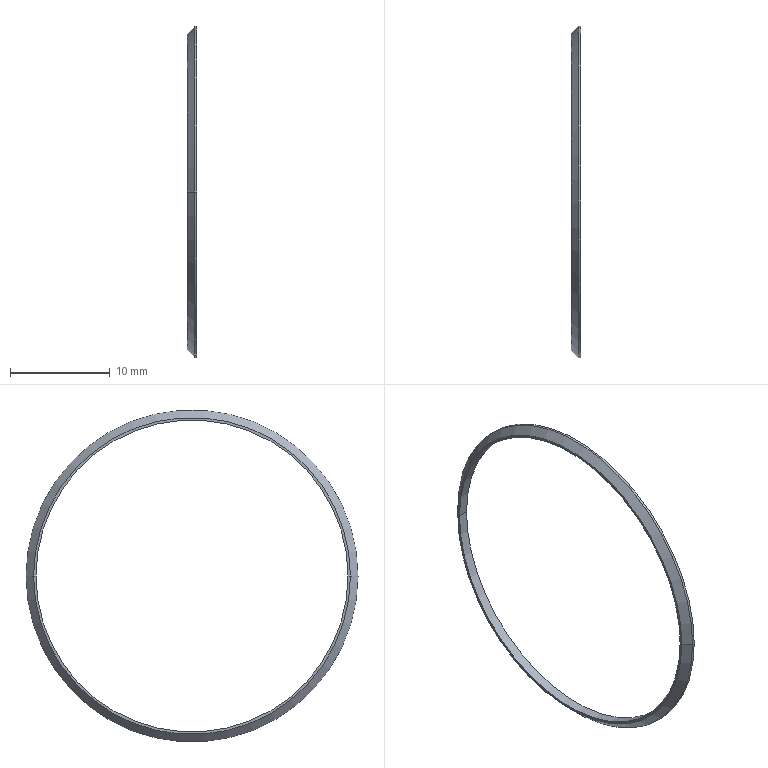Part | STEP file | BREP_7 | 1 solid | 10 faces | box 1 x 33.32 x 33.32 mm | volume 72.205 mm3 | plane 4 | cylinder 4 | cone 2 | commonest cylinder face diameters 31.311 x2 33.32 x2
STEP:
#1=CARTESIAN_POINT('',(0.,0.,0.));
#2=DIRECTION('',(0.,0.,1.));
#3=DIRECTION('',(1.,0.,0.));
#4=AXIS2_PLACEMENT_3D('',#1,#2,#3);
#5=CARTESIAN_POINT('',(-61.38,-16.66,0.));
#6=VERTEX_POINT('',#5);
#7=CARTESIAN_POINT('',(-61.38,-15.656,0.));
#8=VERTEX_POINT('',#7);
#9=CARTESIAN_POINT('',(-61.38,-16.66,0.));
#10=DIRECTION('',(0.,1.,0.));
#11=VECTOR('',#10,1.);
#12=LINE('',#9,#11);
#13=CARTESIAN_POINT('',(-61.38,0.,-16.158));
#14=DIRECTION('',(1.,0.,0.));
#15=DIRECTION('',(0.,-1.,0.));
#16=AXIS2_PLACEMENT_3D('',#13,#14,#15);
#17=PLANE('',#16);
#18=CARTESIAN_POINT('',(16.66,-16.158));
#19=DIRECTION('',(-1.,0.));
#20=VECTOR('',#19,1.);
#21=LINE('',#18,#20);
#22=(GEOMETRIC_REPRESENTATION_CONTEXT(2)PARAMETRIC_REPRESENTATION_CONTEXT()REPRESENTATION_CONTEXT('',''));
#23=DEFINITIONAL_REPRESENTATION('',(#21),#22);
#24=PCURVE('',#17,#23);
#25=CARTESIAN_POINT('',(-61.38,0.,16.158));
#26=DIRECTION('',(1.,0.,0.));
#27=DIRECTION('',(0.,1.,0.));
#28=AXIS2_PLACEMENT_3D('',#25,#26,#27);
#29=PLANE('',#28);
#30=CARTESIAN_POINT('',(-16.66,-16.158));
#31=DIRECTION('',(1.,0.));
#32=VECTOR('',#31,1.);
#33=LINE('',#30,#32);
#34=(GEOMETRIC_REPRESENTATION_CONTEXT(2)PARAMETRIC_REPRESENTATION_CONTEXT()REPRESENTATION_CONTEXT('',''));
#35=DEFINITIONAL_REPRESENTATION('',(#33),#34);
#36=PCURVE('',#29,#35);
#37=SURFACE_CURVE('',#12,(#24,#36),.PCURVE_S1.);
#38=EDGE_CURVE('',#6,#8,#37,.T.);
#39=ORIENTED_EDGE('',*,*,#38,.T.);
#40=CARTESIAN_POINT('',(-61.38,15.656,0.));
#41=VERTEX_POINT('',#40);
#42=CARTESIAN_POINT('',(-61.38,0.,0.));
#43=DIRECTION('',(-1.,0.,0.));
#44=DIRECTION('',(0.,1.,0.));
#45=AXIS2_PLACEMENT_3D('',#42,#43,#44);
#46=CIRCLE('',#45,15.656);
#47=CARTESIAN_POINT('',(-15.656,-16.158));
#48=CARTESIAN_POINT('',(-15.656,10.959));
#49=CARTESIAN_POINT('',(7.828,-2.6));
#50=CARTESIAN_POINT('',(31.311,-16.158));
#51=CARTESIAN_POINT('',(7.828,-29.716));
#52=CARTESIAN_POINT('',(-15.656,-43.274));
#53=CARTESIAN_POINT('',(-15.656,-16.158));
#54=(BOUNDED_CURVE()B_SPLINE_CURVE(2,(#47,#48,#49,#50,#51,#52,#53),.UNSPECIFIED.,.T.,.F.)B_SPLINE_CURVE_WITH_KNOTS((1,2,2,2,2,1),(-2.094,0.,2.094,4.189,6.283,8.378),.UNSPECIFIED.)CURVE()GEOMETRIC_REPRESENTATION_ITEM()RATIONAL_B_SPLINE_CURVE((1.,0.5,1.,0.5,1.,0.5,1.))REPRESENTATION_ITEM(''));
#55=(GEOMETRIC_REPRESENTATION_CONTEXT(2)PARAMETRIC_REPRESENTATION_CONTEXT()REPRESENTATION_CONTEXT('',''));
#56=DEFINITIONAL_REPRESENTATION('',(#54),#55);
#57=PCURVE('',#17,#56);
#58=CARTESIAN_POINT('',(-61.88,0.,0.));
#59=DIRECTION('',(1.,0.,0.));
#60=DIRECTION('',(0.,1.,0.));
#61=AXIS2_PLACEMENT_3D('',#58,#59,#60);
#62=CYLINDRICAL_SURFACE('',#61,15.656);
#63=CARTESIAN_POINT('',(6.283,0.5));
#64=DIRECTION('',(-1.,0.));
#65=VECTOR('',#64,1.);
#66=LINE('',#63,#65);
#67=(GEOMETRIC_REPRESENTATION_CONTEXT(2)PARAMETRIC_REPRESENTATION_CONTEXT()REPRESENTATION_CONTEXT('',''));
#68=DEFINITIONAL_REPRESENTATION('',(#66),#67);
#69=PCURVE('',#62,#68);
#70=SURFACE_CURVE('',#46,(#57,#69),.PCURVE_S1.);
#71=EDGE_CURVE('',#41,#8,#70,.T.);
#72=ORIENTED_EDGE('',*,*,#71,.F.);
#73=CARTESIAN_POINT('',(-61.38,16.66,0.));
#74=VERTEX_POINT('',#73);
#75=CARTESIAN_POINT('',(-61.38,16.66,0.));
#76=DIRECTION('',(0.,-1.,0.));
#77=VECTOR('',#76,1.);
#78=LINE('',#75,#77);
#79=CARTESIAN_POINT('',(-16.66,-16.158));
#80=DIRECTION('',(1.,0.));
#81=VECTOR('',#80,1.);
#82=LINE('',#79,#81);
#83=(GEOMETRIC_REPRESENTATION_CONTEXT(2)PARAMETRIC_REPRESENTATION_CONTEXT()REPRESENTATION_CONTEXT('',''));
#84=DEFINITIONAL_REPRESENTATION('',(#82),#83);
#85=PCURVE('',#17,#84);
#86=CARTESIAN_POINT('',(16.66,-16.158));
#87=DIRECTION('',(-1.,0.));
#88=VECTOR('',#87,1.);
#89=LINE('',#86,#88);
#90=(GEOMETRIC_REPRESENTATION_CONTEXT(2)PARAMETRIC_REPRESENTATION_CONTEXT()REPRESENTATION_CONTEXT('',''));
#91=DEFINITIONAL_REPRESENTATION('',(#89),#90);
#92=PCURVE('',#29,#91);
#93=SURFACE_CURVE('',#78,(#85,#92),.PCURVE_S1.);
#94=EDGE_CURVE('',#74,#41,#93,.T.);
#95=ORIENTED_EDGE('',*,*,#94,.F.);
#96=CARTESIAN_POINT('',(-61.38,0.,0.));
#97=DIRECTION('',(1.,0.,0.));
#98=DIRECTION('',(0.,-1.,0.));
#99=AXIS2_PLACEMENT_3D('',#96,#97,#98);
#100=CIRCLE('',#99,16.66);
#101=CARTESIAN_POINT('',(0.,-16.158));
#102=DIRECTION('',(1.,0.));
#103=AXIS2_PLACEMENT_2D('',#101,#102);
#104=CIRCLE('',#103,16.66);
#105=(GEOMETRIC_REPRESENTATION_CONTEXT(2)PARAMETRIC_REPRESENTATION_CONTEXT()REPRESENTATION_CONTEXT('',''));
#106=DEFINITIONAL_REPRESENTATION('',(#104),#105);
#107=PCURVE('',#17,#106);
#108=CARTESIAN_POINT('',(-61.5,0.,0.));
#109=DIRECTION('',(-1.,0.,0.));
#110=DIRECTION('',(0.,1.,0.));
#111=AXIS2_PLACEMENT_3D('',#108,#109,#110);
#112=CYLINDRICAL_SURFACE('',#111,16.66);
#113=CARTESIAN_POINT('',(3.142,-0.12));
#114=DIRECTION('',(-1.,0.));
#115=VECTOR('',#114,1.);
#116=LINE('',#113,#115);
#117=(GEOMETRIC_REPRESENTATION_CONTEXT(2)PARAMETRIC_REPRESENTATION_CONTEXT()REPRESENTATION_CONTEXT('',''));
#118=DEFINITIONAL_REPRESENTATION('',(#116),#117);
#119=PCURVE('',#112,#118);
#120=SURFACE_CURVE('',#100,(#107,#119),.PCURVE_S1.);
#121=EDGE_CURVE('',#6,#74,#120,.T.);
#122=ORIENTED_EDGE('',*,*,#121,.F.);
#123=EDGE_LOOP('',(#39,#72,#95,#122));
#124=FACE_BOUND('',#123,.F.);
#125=ADVANCED_FACE('',(#124),#17,.T.);
#126=CARTESIAN_POINT('',(-61.38,0.,0.));
#127=DIRECTION('',(-1.,0.,0.));
#128=DIRECTION('',(0.,-1.,0.));
#129=AXIS2_PLACEMENT_3D('',#126,#127,#128);
#130=CIRCLE('',#129,15.656);
#131=CARTESIAN_POINT('',(-15.656,-16.158));
#132=CARTESIAN_POINT('',(-15.656,10.959));
#133=CARTESIAN_POINT('',(7.828,-2.6));
#134=CARTESIAN_POINT('',(31.311,-16.158));
#135=CARTESIAN_POINT('',(7.828,-29.716));
#136=CARTESIAN_POINT('',(-15.656,-43.274));
#137=CARTESIAN_POINT('',(-15.656,-16.158));
#138=(BOUNDED_CURVE()B_SPLINE_CURVE(2,(#131,#132,#133,#134,#135,#136,#137),.UNSPECIFIED.,.T.,.F.)B_SPLINE_CURVE_WITH_KNOTS((1,2,2,2,2,1),(-2.094,0.,2.094,4.189,6.283,8.378),.UNSPECIFIED.)CURVE()GEOMETRIC_REPRESENTATION_ITEM()RATIONAL_B_SPLINE_CURVE((1.,0.5,1.,0.5,1.,0.5,1.))REPRESENTATION_ITEM(''));
#139=(GEOMETRIC_REPRESENTATION_CONTEXT(2)PARAMETRIC_REPRESENTATION_CONTEXT()REPRESENTATION_CONTEXT('',''));
#140=DEFINITIONAL_REPRESENTATION('',(#138),#139);
#141=PCURVE('',#29,#140);
#142=CARTESIAN_POINT('',(-61.88,0.,0.));
#143=DIRECTION('',(1.,0.,0.));
#144=DIRECTION('',(0.,-1.,0.));
#145=AXIS2_PLACEMENT_3D('',#142,#143,#144);
#146=CYLINDRICAL_SURFACE('',#145,15.656);
#147=CARTESIAN_POINT('',(6.283,0.5));
#148=DIRECTION('',(-1.,0.));
#149=VECTOR('',#148,1.);
#150=LINE('',#147,#149);
#151=(GEOMETRIC_REPRESENTATION_CONTEXT(2)PARAMETRIC_REPRESENTATION_CONTEXT()REPRESENTATION_CONTEXT('',''));
#152=DEFINITIONAL_REPRESENTATION('',(#150),#151);
#153=PCURVE('',#146,#152);
#154=SURFACE_CURVE('',#130,(#141,#153),.PCURVE_S1.);
#155=EDGE_CURVE('',#8,#41,#154,.T.);
#156=ORIENTED_EDGE('',*,*,#155,.F.);
#157=ORIENTED_EDGE('',*,*,#38,.F.);
#158=CARTESIAN_POINT('',(-61.38,0.,0.));
#159=DIRECTION('',(1.,0.,0.));
#160=DIRECTION('',(0.,1.,0.));
#161=AXIS2_PLACEMENT_3D('',#158,#159,#160);
#162=CIRCLE('',#161,16.66);
#163=CARTESIAN_POINT('',(0.,-16.158));
#164=DIRECTION('',(1.,0.));
#165=AXIS2_PLACEMENT_2D('',#163,#164);
#166=CIRCLE('',#165,16.66);
#167=(GEOMETRIC_REPRESENTATION_CONTEXT(2)PARAMETRIC_REPRESENTATION_CONTEXT()REPRESENTATION_CONTEXT('',''));
#168=DEFINITIONAL_REPRESENTATION('',(#166),#167);
#169=PCURVE('',#29,#168);
#170=CARTESIAN_POINT('',(-61.5,0.,0.));
#171=DIRECTION('',(-1.,0.,0.));
#172=DIRECTION('',(0.,-1.,0.));
#173=AXIS2_PLACEMENT_3D('',#170,#171,#172);
#174=CYLINDRICAL_SURFACE('',#173,16.66);
#175=CARTESIAN_POINT('',(3.142,-0.12));
#176=DIRECTION('',(-1.,0.));
#177=VECTOR('',#176,1.);
#178=LINE('',#175,#177);
#179=(GEOMETRIC_REPRESENTATION_CONTEXT(2)PARAMETRIC_REPRESENTATION_CONTEXT()REPRESENTATION_CONTEXT('',''));
#180=DEFINITIONAL_REPRESENTATION('',(#178),#179);
#181=PCURVE('',#174,#180);
#182=SURFACE_CURVE('',#162,(#169,#181),.PCURVE_S1.);
#183=EDGE_CURVE('',#74,#6,#182,.T.);
#184=ORIENTED_EDGE('',*,*,#183,.F.);
#185=ORIENTED_EDGE('',*,*,#94,.T.);
#186=EDGE_LOOP('',(#156,#157,#184,#185));
#187=FACE_BOUND('',#186,.F.);
#188=ADVANCED_FACE('',(#187),#29,.T.);
#189=CARTESIAN_POINT('',(-62.38,15.656,0.));
#190=VERTEX_POINT('',#189);
#191=CARTESIAN_POINT('',(-62.38,-15.656,0.));
#192=VERTEX_POINT('',#191);
#193=CARTESIAN_POINT('',(-62.38,0.,0.));
#194=DIRECTION('',(1.,0.,0.));
#195=DIRECTION('',(0.,1.,0.));
#196=AXIS2_PLACEMENT_3D('',#193,#194,#195);
#197=CIRCLE('',#196,15.656);
#198=CARTESIAN_POINT('',(3.142,-0.5));
#199=DIRECTION('',(1.,0.));
#200=VECTOR('',#199,1.);
#201=LINE('',#198,#200);
#202=(GEOMETRIC_REPRESENTATION_CONTEXT(2)PARAMETRIC_REPRESENTATION_CONTEXT()REPRESENTATION_CONTEXT('',''));
#203=DEFINITIONAL_REPRESENTATION('',(#201),#202);
#204=PCURVE('',#146,#203);
#205=CARTESIAN_POINT('',(-62.38,0.,15.778));
#206=DIRECTION('',(1.,0.,0.));
#207=DIRECTION('',(0.,1.,0.));
#208=AXIS2_PLACEMENT_3D('',#205,#206,#207);
#209=PLANE('',#208);
#210=CARTESIAN_POINT('',(0.,-15.778));
#211=DIRECTION('',(1.,0.));
#212=AXIS2_PLACEMENT_2D('',#210,#211);
#213=CIRCLE('',#212,15.656);
#214=(GEOMETRIC_REPRESENTATION_CONTEXT(2)PARAMETRIC_REPRESENTATION_CONTEXT()REPRESENTATION_CONTEXT('',''));
#215=DEFINITIONAL_REPRESENTATION('',(#213),#214);
#216=PCURVE('',#209,#215);
#217=SURFACE_CURVE('',#197,(#204,#216),.PCURVE_S1.);
#218=EDGE_CURVE('',#190,#192,#217,.T.);
#219=ORIENTED_EDGE('',*,*,#218,.T.);
#220=CARTESIAN_POINT('',(-61.38,-15.656,0.));
#221=DIRECTION('',(-1.,0.,0.));
#222=VECTOR('',#221,1.);
#223=LINE('',#220,#222);
#224=CARTESIAN_POINT('',(6.283,0.5));
#225=DIRECTION('',(0.,-1.));
#226=VECTOR('',#225,1.);
#227=LINE('',#224,#226);
#228=(GEOMETRIC_REPRESENTATION_CONTEXT(2)PARAMETRIC_REPRESENTATION_CONTEXT()REPRESENTATION_CONTEXT('',''));
#229=DEFINITIONAL_REPRESENTATION('',(#227),#228);
#230=PCURVE('',#146,#229);
#231=CARTESIAN_POINT('',(3.142,0.5));
#232=DIRECTION('',(0.,-1.));
#233=VECTOR('',#232,1.);
#234=LINE('',#231,#233);
#235=(GEOMETRIC_REPRESENTATION_CONTEXT(2)PARAMETRIC_REPRESENTATION_CONTEXT()REPRESENTATION_CONTEXT('',''));
#236=DEFINITIONAL_REPRESENTATION('',(#234),#235);
#237=PCURVE('',#62,#236);
#238=SURFACE_CURVE('',#223,(#230,#237),.PCURVE_S1.);
#239=EDGE_CURVE('',#8,#192,#238,.T.);
#240=ORIENTED_EDGE('',*,*,#239,.F.);
#241=ORIENTED_EDGE('',*,*,#155,.T.);
#242=CARTESIAN_POINT('',(-61.38,15.656,0.));
#243=DIRECTION('',(-1.,0.,0.));
#244=VECTOR('',#243,1.);
#245=LINE('',#242,#244);
#246=CARTESIAN_POINT('',(3.142,0.5));
#247=DIRECTION('',(0.,-1.));
#248=VECTOR('',#247,1.);
#249=LINE('',#246,#248);
#250=(GEOMETRIC_REPRESENTATION_CONTEXT(2)PARAMETRIC_REPRESENTATION_CONTEXT()REPRESENTATION_CONTEXT('',''));
#251=DEFINITIONAL_REPRESENTATION('',(#249),#250);
#252=PCURVE('',#146,#251);
#253=CARTESIAN_POINT('',(6.283,0.5));
#254=DIRECTION('',(0.,-1.));
#255=VECTOR('',#254,1.);
#256=LINE('',#253,#255);
#257=(GEOMETRIC_REPRESENTATION_CONTEXT(2)PARAMETRIC_REPRESENTATION_CONTEXT()REPRESENTATION_CONTEXT('',''));
#258=DEFINITIONAL_REPRESENTATION('',(#256),#257);
#259=PCURVE('',#62,#258);
#260=SURFACE_CURVE('',#245,(#252,#259),.PCURVE_S1.);
#261=EDGE_CURVE('',#41,#190,#260,.T.);
#262=ORIENTED_EDGE('',*,*,#261,.T.);
#263=EDGE_LOOP('',(#219,#240,#241,#262));
#264=FACE_BOUND('',#263,.F.);
#265=ADVANCED_FACE('',(#264),#146,.F.);
#266=CARTESIAN_POINT('',(-62.38,-15.9,0.));
#267=VERTEX_POINT('',#266);
#268=CARTESIAN_POINT('',(-62.38,15.9,0.));
#269=VERTEX_POINT('',#268);
#270=CARTESIAN_POINT('',(-62.38,0.,0.));
#271=DIRECTION('',(-1.,0.,0.));
#272=DIRECTION('',(0.,-1.,0.));
#273=AXIS2_PLACEMENT_3D('',#270,#271,#272);
#274=CIRCLE('',#273,15.9);
#275=CARTESIAN_POINT('',(-15.9,-15.778));
#276=CARTESIAN_POINT('',(-15.9,11.762));
#277=CARTESIAN_POINT('',(7.95,-2.008));
#278=CARTESIAN_POINT('',(31.8,-15.778));
#279=CARTESIAN_POINT('',(7.95,-29.548));
#280=CARTESIAN_POINT('',(-15.9,-43.317));
#281=CARTESIAN_POINT('',(-15.9,-15.778));
#282=(BOUNDED_CURVE()B_SPLINE_CURVE(2,(#275,#276,#277,#278,#279,#280,#281),.UNSPECIFIED.,.T.,.F.)B_SPLINE_CURVE_WITH_KNOTS((1,2,2,2,2,1),(-2.094,0.,2.094,4.189,6.283,8.378),.UNSPECIFIED.)CURVE()GEOMETRIC_REPRESENTATION_ITEM()RATIONAL_B_SPLINE_CURVE((1.,0.5,1.,0.5,1.,0.5,1.))REPRESENTATION_ITEM(''));
#283=(GEOMETRIC_REPRESENTATION_CONTEXT(2)PARAMETRIC_REPRESENTATION_CONTEXT()REPRESENTATION_CONTEXT('',''));
#284=DEFINITIONAL_REPRESENTATION('',(#282),#283);
#285=PCURVE('',#209,#284);
#286=CARTESIAN_POINT('',(-62.,0.,0.));
#287=DIRECTION('',(1.,0.,0.));
#288=DIRECTION('',(0.,1.,0.));
#289=AXIS2_PLACEMENT_3D('',#286,#287,#288);
#290=CONICAL_SURFACE('',#289,16.28,0.7854);
#291=CARTESIAN_POINT('',(3.142,-0.38));
#292=DIRECTION('',(-1.,0.));
#293=VECTOR('',#292,1.);
#294=LINE('',#291,#293);
#295=(GEOMETRIC_REPRESENTATION_CONTEXT(2)PARAMETRIC_REPRESENTATION_CONTEXT()REPRESENTATION_CONTEXT('',''));
#296=DEFINITIONAL_REPRESENTATION('',(#294),#295);
#297=PCURVE('',#290,#296);
#298=SURFACE_CURVE('',#274,(#285,#297),.PCURVE_S1.);
#299=EDGE_CURVE('',#267,#269,#298,.T.);
#300=ORIENTED_EDGE('',*,*,#299,.F.);
#301=CARTESIAN_POINT('',(-62.38,-15.656,0.));
#302=DIRECTION('',(0.,-1.,0.));
#303=VECTOR('',#302,1.);
#304=LINE('',#301,#303);
#305=CARTESIAN_POINT('',(-15.656,-15.778));
#306=DIRECTION('',(-1.,0.));
#307=VECTOR('',#306,1.);
#308=LINE('',#305,#307);
#309=(GEOMETRIC_REPRESENTATION_CONTEXT(2)PARAMETRIC_REPRESENTATION_CONTEXT()REPRESENTATION_CONTEXT('',''));
#310=DEFINITIONAL_REPRESENTATION('',(#308),#309);
#311=PCURVE('',#209,#310);
#312=CARTESIAN_POINT('',(-62.38,0.,-15.778));
#313=DIRECTION('',(1.,0.,0.));
#314=DIRECTION('',(0.,-1.,0.));
#315=AXIS2_PLACEMENT_3D('',#312,#313,#314);
#316=PLANE('',#315);
#317=CARTESIAN_POINT('',(15.656,-15.778));
#318=DIRECTION('',(1.,0.));
#319=VECTOR('',#318,1.);
#320=LINE('',#317,#319);
#321=(GEOMETRIC_REPRESENTATION_CONTEXT(2)PARAMETRIC_REPRESENTATION_CONTEXT()REPRESENTATION_CONTEXT('',''));
#322=DEFINITIONAL_REPRESENTATION('',(#320),#321);
#323=PCURVE('',#316,#322);
#324=SURFACE_CURVE('',#304,(#311,#323),.PCURVE_S1.);
#325=EDGE_CURVE('',#192,#267,#324,.T.);
#326=ORIENTED_EDGE('',*,*,#325,.F.);
#327=ORIENTED_EDGE('',*,*,#218,.F.);
#328=CARTESIAN_POINT('',(-62.38,15.656,0.));
#329=DIRECTION('',(0.,1.,0.));
#330=VECTOR('',#329,1.);
#331=LINE('',#328,#330);
#332=CARTESIAN_POINT('',(15.656,-15.778));
#333=DIRECTION('',(1.,0.));
#334=VECTOR('',#333,1.);
#335=LINE('',#332,#334);
#336=(GEOMETRIC_REPRESENTATION_CONTEXT(2)PARAMETRIC_REPRESENTATION_CONTEXT()REPRESENTATION_CONTEXT('',''));
#337=DEFINITIONAL_REPRESENTATION('',(#335),#336);
#338=PCURVE('',#209,#337);
#339=CARTESIAN_POINT('',(-15.656,-15.778));
#340=DIRECTION('',(-1.,0.));
#341=VECTOR('',#340,1.);
#342=LINE('',#339,#341);
#343=(GEOMETRIC_REPRESENTATION_CONTEXT(2)PARAMETRIC_REPRESENTATION_CONTEXT()REPRESENTATION_CONTEXT('',''));
#344=DEFINITIONAL_REPRESENTATION('',(#342),#343);
#345=PCURVE('',#316,#344);
#346=SURFACE_CURVE('',#331,(#338,#345),.PCURVE_S1.);
#347=EDGE_CURVE('',#190,#269,#346,.T.);
#348=ORIENTED_EDGE('',*,*,#347,.T.);
#349=EDGE_LOOP('',(#300,#326,#327,#348));
#350=FACE_BOUND('',#349,.F.);
#351=ADVANCED_FACE('',(#350),#209,.F.);
#352=CARTESIAN_POINT('',(-61.62,16.66,0.));
#353=VERTEX_POINT('',#352);
#354=CARTESIAN_POINT('',(-62.38,15.9,0.));
#355=DIRECTION('',(0.7071,0.7071,0.));
#356=VECTOR('',#355,1.);
#357=LINE('',#354,#356);
#358=CARTESIAN_POINT('',(0.,-0.3799));
#359=DIRECTION('',(0.,1.));
#360=VECTOR('',#359,1.);
#361=LINE('',#358,#360);
#362=(GEOMETRIC_REPRESENTATION_CONTEXT(2)PARAMETRIC_REPRESENTATION_CONTEXT()REPRESENTATION_CONTEXT('',''));
#363=DEFINITIONAL_REPRESENTATION('',(#361),#362);
#364=PCURVE('',#290,#363);
#365=CARTESIAN_POINT('',(-62.,0.,0.));
#366=DIRECTION('',(1.,0.,0.));
#367=DIRECTION('',(0.,-1.,0.));
#368=AXIS2_PLACEMENT_3D('',#365,#366,#367);
#369=CONICAL_SURFACE('',#368,16.28,0.7854);
#370=CARTESIAN_POINT('',(3.142,-0.3799));
#371=DIRECTION('',(0.,1.));
#372=VECTOR('',#371,1.);
#373=LINE('',#370,#372);
#374=(GEOMETRIC_REPRESENTATION_CONTEXT(2)PARAMETRIC_REPRESENTATION_CONTEXT()REPRESENTATION_CONTEXT('',''));
#375=DEFINITIONAL_REPRESENTATION('',(#373),#374);
#376=PCURVE('',#369,#375);
#377=SURFACE_CURVE('',#357,(#364,#376),.PCURVE_S1.);
#378=EDGE_CURVE('',#269,#353,#377,.T.);
#379=ORIENTED_EDGE('',*,*,#378,.F.);
#380=ORIENTED_EDGE('',*,*,#299,.F.);
#381=CARTESIAN_POINT('',(-61.62,-16.66,0.));
#382=VERTEX_POINT('',#381);
#383=CARTESIAN_POINT('',(-62.38,-15.9,0.));
#384=DIRECTION('',(0.7071,-0.7071,0.));
#385=VECTOR('',#384,1.);
#386=LINE('',#383,#385);
#387=CARTESIAN_POINT('',(3.142,-0.3799));
#388=DIRECTION('',(0.,1.));
#389=VECTOR('',#388,1.);
#390=LINE('',#387,#389);
#391=(GEOMETRIC_REPRESENTATION_CONTEXT(2)PARAMETRIC_REPRESENTATION_CONTEXT()REPRESENTATION_CONTEXT('',''));
#392=DEFINITIONAL_REPRESENTATION('',(#390),#391);
#393=PCURVE('',#290,#392);
#394=CARTESIAN_POINT('',(0.,-0.3799));
#395=DIRECTION('',(0.,1.));
#396=VECTOR('',#395,1.);
#397=LINE('',#394,#396);
#398=(GEOMETRIC_REPRESENTATION_CONTEXT(2)PARAMETRIC_REPRESENTATION_CONTEXT()REPRESENTATION_CONTEXT('',''));
#399=DEFINITIONAL_REPRESENTATION('',(#397),#398);
#400=PCURVE('',#369,#399);
#401=SURFACE_CURVE('',#386,(#393,#400),.PCURVE_S1.);
#402=EDGE_CURVE('',#267,#382,#401,.T.);
#403=ORIENTED_EDGE('',*,*,#402,.T.);
#404=CARTESIAN_POINT('',(-61.62,0.,0.));
#405=DIRECTION('',(1.,0.,0.));
#406=DIRECTION('',(0.,1.,0.));
#407=AXIS2_PLACEMENT_3D('',#404,#405,#406);
#408=CIRCLE('',#407,16.66);
#409=CARTESIAN_POINT('',(0.,0.3801));
#410=DIRECTION('',(1.,0.));
#411=VECTOR('',#410,1.);
#412=LINE('',#409,#411);
#413=(GEOMETRIC_REPRESENTATION_CONTEXT(2)PARAMETRIC_REPRESENTATION_CONTEXT()REPRESENTATION_CONTEXT('',''));
#414=DEFINITIONAL_REPRESENTATION('',(#412),#413);
#415=PCURVE('',#290,#414);
#416=CARTESIAN_POINT('',(3.142,0.12));
#417=DIRECTION('',(-1.,0.));
#418=VECTOR('',#417,1.);
#419=LINE('',#416,#418);
#420=(GEOMETRIC_REPRESENTATION_CONTEXT(2)PARAMETRIC_REPRESENTATION_CONTEXT()REPRESENTATION_CONTEXT('',''));
#421=DEFINITIONAL_REPRESENTATION('',(#419),#420);
#422=PCURVE('',#174,#421);
#423=SURFACE_CURVE('',#408,(#415,#422),.PCURVE_S1.);
#424=EDGE_CURVE('',#353,#382,#423,.T.);
#425=ORIENTED_EDGE('',*,*,#424,.F.);
#426=EDGE_LOOP('',(#379,#380,#403,#425));
#427=FACE_BOUND('',#426,.T.);
#428=ADVANCED_FACE('',(#427),#290,.T.);
#429=CARTESIAN_POINT('',(-61.62,16.66,0.));
#430=DIRECTION('',(1.,0.,0.));
#431=VECTOR('',#430,1.);
#432=LINE('',#429,#431);
#433=CARTESIAN_POINT('',(3.142,0.12));
#434=DIRECTION('',(0.,-1.));
#435=VECTOR('',#434,1.);
#436=LINE('',#433,#435);
#437=(GEOMETRIC_REPRESENTATION_CONTEXT(2)PARAMETRIC_REPRESENTATION_CONTEXT()REPRESENTATION_CONTEXT('',''));
#438=DEFINITIONAL_REPRESENTATION('',(#436),#437);
#439=PCURVE('',#174,#438);
#440=CARTESIAN_POINT('',(0.,0.12));
#441=DIRECTION('',(0.,-1.));
#442=VECTOR('',#441,1.);
#443=LINE('',#440,#442);
#444=(GEOMETRIC_REPRESENTATION_CONTEXT(2)PARAMETRIC_REPRESENTATION_CONTEXT()REPRESENTATION_CONTEXT('',''));
#445=DEFINITIONAL_REPRESENTATION('',(#443),#444);
#446=PCURVE('',#112,#445);
#447=SURFACE_CURVE('',#432,(#439,#446),.PCURVE_S1.);
#448=EDGE_CURVE('',#353,#74,#447,.T.);
#449=ORIENTED_EDGE('',*,*,#448,.F.);
#450=ORIENTED_EDGE('',*,*,#424,.T.);
#451=CARTESIAN_POINT('',(-61.62,-16.66,0.));
#452=DIRECTION('',(1.,0.,0.));
#453=VECTOR('',#452,1.);
#454=LINE('',#451,#453);
#455=CARTESIAN_POINT('',(0.,0.12));
#456=DIRECTION('',(0.,-1.));
#457=VECTOR('',#456,1.);
#458=LINE('',#455,#457);
#459=(GEOMETRIC_REPRESENTATION_CONTEXT(2)PARAMETRIC_REPRESENTATION_CONTEXT()REPRESENTATION_CONTEXT('',''));
#460=DEFINITIONAL_REPRESENTATION('',(#458),#459);
#461=PCURVE('',#174,#460);
#462=CARTESIAN_POINT('',(3.142,0.12));
#463=DIRECTION('',(0.,-1.));
#464=VECTOR('',#463,1.);
#465=LINE('',#462,#464);
#466=(GEOMETRIC_REPRESENTATION_CONTEXT(2)PARAMETRIC_REPRESENTATION_CONTEXT()REPRESENTATION_CONTEXT('',''));
#467=DEFINITIONAL_REPRESENTATION('',(#465),#466);
#468=PCURVE('',#112,#467);
#469=SURFACE_CURVE('',#454,(#461,#468),.PCURVE_S1.);
#470=EDGE_CURVE('',#382,#6,#469,.T.);
#471=ORIENTED_EDGE('',*,*,#470,.T.);
#472=ORIENTED_EDGE('',*,*,#183,.F.);
#473=EDGE_LOOP('',(#449,#450,#471,#472));
#474=FACE_BOUND('',#473,.T.);
#475=ADVANCED_FACE('',(#474),#174,.T.);
#476=CARTESIAN_POINT('',(-61.62,0.,0.));
#477=DIRECTION('',(1.,0.,0.));
#478=DIRECTION('',(0.,-1.,0.));
#479=AXIS2_PLACEMENT_3D('',#476,#477,#478);
#480=CIRCLE('',#479,16.66);
#481=CARTESIAN_POINT('',(3.142,0.12));
#482=DIRECTION('',(-1.,0.));
#483=VECTOR('',#482,1.);
#484=LINE('',#481,#483);
#485=(GEOMETRIC_REPRESENTATION_CONTEXT(2)PARAMETRIC_REPRESENTATION_CONTEXT()REPRESENTATION_CONTEXT('',''));
#486=DEFINITIONAL_REPRESENTATION('',(#484),#485);
#487=PCURVE('',#112,#486);
#488=CARTESIAN_POINT('',(0.,0.3801));
#489=DIRECTION('',(1.,0.));
#490=VECTOR('',#489,1.);
#491=LINE('',#488,#490);
#492=(GEOMETRIC_REPRESENTATION_CONTEXT(2)PARAMETRIC_REPRESENTATION_CONTEXT()REPRESENTATION_CONTEXT('',''));
#493=DEFINITIONAL_REPRESENTATION('',(#491),#492);
#494=PCURVE('',#369,#493);
#495=SURFACE_CURVE('',#480,(#487,#494),.PCURVE_S1.);
#496=EDGE_CURVE('',#382,#353,#495,.T.);
#497=ORIENTED_EDGE('',*,*,#496,.T.);
#498=ORIENTED_EDGE('',*,*,#448,.T.);
#499=ORIENTED_EDGE('',*,*,#121,.F.);
#500=ORIENTED_EDGE('',*,*,#470,.F.);
#501=EDGE_LOOP('',(#497,#498,#499,#500));
#502=FACE_BOUND('',#501,.T.);
#503=ADVANCED_FACE('',(#502),#112,.T.);
#504=CARTESIAN_POINT('',(-62.38,0.,0.));
#505=DIRECTION('',(-1.,0.,0.));
#506=DIRECTION('',(0.,1.,0.));
#507=AXIS2_PLACEMENT_3D('',#504,#505,#506);
#508=CIRCLE('',#507,15.9);
#509=CARTESIAN_POINT('',(3.142,-0.38));
#510=DIRECTION('',(-1.,0.));
#511=VECTOR('',#510,1.);
#512=LINE('',#509,#511);
#513=(GEOMETRIC_REPRESENTATION_CONTEXT(2)PARAMETRIC_REPRESENTATION_CONTEXT()REPRESENTATION_CONTEXT('',''));
#514=DEFINITIONAL_REPRESENTATION('',(#512),#513);
#515=PCURVE('',#369,#514);
#516=CARTESIAN_POINT('',(-15.9,-15.778));
#517=CARTESIAN_POINT('',(-15.9,11.762));
#518=CARTESIAN_POINT('',(7.95,-2.008));
#519=CARTESIAN_POINT('',(31.8,-15.778));
#520=CARTESIAN_POINT('',(7.95,-29.548));
#521=CARTESIAN_POINT('',(-15.9,-43.317));
#522=CARTESIAN_POINT('',(-15.9,-15.778));
#523=(BOUNDED_CURVE()B_SPLINE_CURVE(2,(#516,#517,#518,#519,#520,#521,#522),.UNSPECIFIED.,.T.,.F.)B_SPLINE_CURVE_WITH_KNOTS((1,2,2,2,2,1),(-2.094,0.,2.094,4.189,6.283,8.378),.UNSPECIFIED.)CURVE()GEOMETRIC_REPRESENTATION_ITEM()RATIONAL_B_SPLINE_CURVE((1.,0.5,1.,0.5,1.,0.5,1.))REPRESENTATION_ITEM(''));
#524=(GEOMETRIC_REPRESENTATION_CONTEXT(2)PARAMETRIC_REPRESENTATION_CONTEXT()REPRESENTATION_CONTEXT('',''));
#525=DEFINITIONAL_REPRESENTATION('',(#523),#524);
#526=PCURVE('',#316,#525);
#527=SURFACE_CURVE('',#508,(#515,#526),.PCURVE_S1.);
#528=EDGE_CURVE('',#269,#267,#527,.T.);
#529=ORIENTED_EDGE('',*,*,#528,.F.);
#530=ORIENTED_EDGE('',*,*,#378,.T.);
#531=ORIENTED_EDGE('',*,*,#496,.F.);
#532=ORIENTED_EDGE('',*,*,#402,.F.);
#533=EDGE_LOOP('',(#529,#530,#531,#532));
#534=FACE_BOUND('',#533,.T.);
#535=ADVANCED_FACE('',(#534),#369,.T.);
#536=ORIENTED_EDGE('',*,*,#325,.T.);
#537=ORIENTED_EDGE('',*,*,#528,.F.);
#538=ORIENTED_EDGE('',*,*,#347,.F.);
#539=CARTESIAN_POINT('',(-62.38,0.,0.));
#540=DIRECTION('',(1.,0.,0.));
#541=DIRECTION('',(0.,-1.,0.));
#542=AXIS2_PLACEMENT_3D('',#539,#540,#541);
#543=CIRCLE('',#542,15.656);
#544=CARTESIAN_POINT('',(0.,-15.778));
#545=DIRECTION('',(1.,0.));
#546=AXIS2_PLACEMENT_2D('',#544,#545);
#547=CIRCLE('',#546,15.656);
#548=(GEOMETRIC_REPRESENTATION_CONTEXT(2)PARAMETRIC_REPRESENTATION_CONTEXT()REPRESENTATION_CONTEXT('',''));
#549=DEFINITIONAL_REPRESENTATION('',(#547),#548);
#550=PCURVE('',#316,#549);
#551=CARTESIAN_POINT('',(3.142,-0.5));
#552=DIRECTION('',(1.,0.));
#553=VECTOR('',#552,1.);
#554=LINE('',#551,#553);
#555=(GEOMETRIC_REPRESENTATION_CONTEXT(2)PARAMETRIC_REPRESENTATION_CONTEXT()REPRESENTATION_CONTEXT('',''));
#556=DEFINITIONAL_REPRESENTATION('',(#554),#555);
#557=PCURVE('',#62,#556);
#558=SURFACE_CURVE('',#543,(#550,#557),.PCURVE_S1.);
#559=EDGE_CURVE('',#192,#190,#558,.T.);
#560=ORIENTED_EDGE('',*,*,#559,.F.);
#561=EDGE_LOOP('',(#536,#537,#538,#560));
#562=FACE_BOUND('',#561,.F.);
#563=ADVANCED_FACE('',(#562),#316,.F.);
#564=ORIENTED_EDGE('',*,*,#239,.T.);
#565=ORIENTED_EDGE('',*,*,#559,.T.);
#566=ORIENTED_EDGE('',*,*,#261,.F.);
#567=ORIENTED_EDGE('',*,*,#71,.T.);
#568=EDGE_LOOP('',(#564,#565,#566,#567));
#569=FACE_BOUND('',#568,.F.);
#570=ADVANCED_FACE('',(#569),#62,.F.);
#571=CLOSED_SHELL('',(#125,#188,#265,#351,#428,#475,#503,#535,#563,#570));
#572=MANIFOLD_SOLID_BREP('',#571);
#573=(LENGTH_UNIT()NAMED_UNIT(*)SI_UNIT(.MILLI.,.METRE.));
#574=UNCERTAINTY_MEASURE_WITH_UNIT(LENGTH_MEASURE(0.00001),#573,'','');
#575=(NAMED_UNIT(*)PLANE_ANGLE_UNIT()SI_UNIT($,.RADIAN.));
#576=(NAMED_UNIT(*)SI_UNIT($,.STERADIAN.)SOLID_ANGLE_UNIT());
#577=(GEOMETRIC_REPRESENTATION_CONTEXT(3)GLOBAL_UNCERTAINTY_ASSIGNED_CONTEXT((#574))GLOBAL_UNIT_ASSIGNED_CONTEXT((#573,#575,#576))REPRESENTATION_CONTEXT('',''));
#578=ADVANCED_BREP_SHAPE_REPRESENTATION('',(#4,#572),#577);